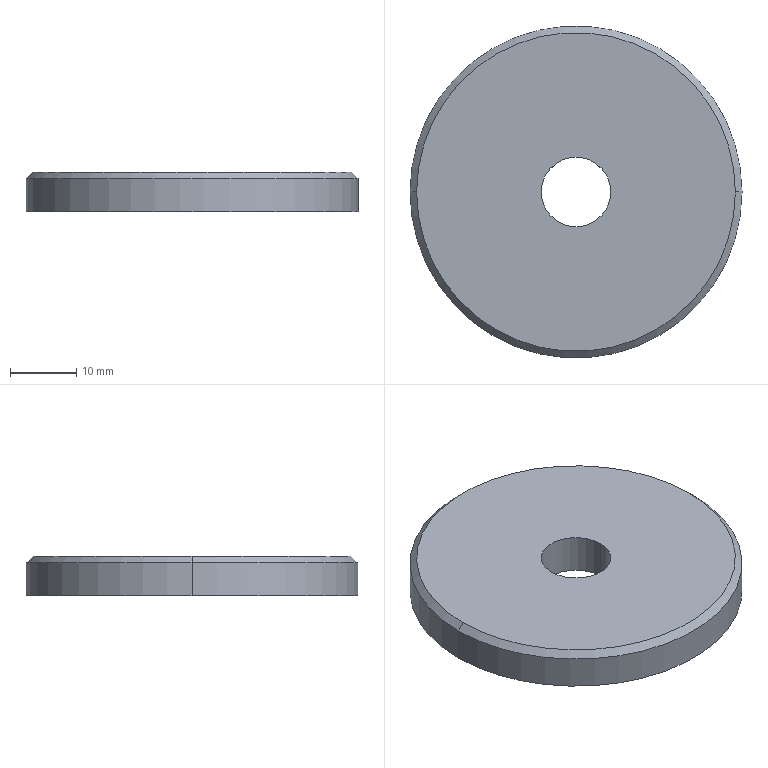Part | SolidWorks | features Chamfer 1, Extrusion 1 | 1 solid | 8 faces | box 50 x 50 x 6 mm | volume 11184 mm3 | cylinder 4 | cone 2 | plane 2 | commonest cylinder face diameters 10.5 x2 50 x2
STEP:
#1=CARTESIAN_POINT('',(24.,0.,6.));
#2=VERTEX_POINT('',#1);
#3=CARTESIAN_POINT('',(-24.,0.,6.));
#4=VERTEX_POINT('',#3);
#5=CARTESIAN_POINT('',(0.,0.,6.));
#6=DIRECTION('',(0.,0.,1.));
#7=DIRECTION('',(1.,0.,0.));
#8=AXIS2_PLACEMENT_3D('',#5,#6,#7);
#9=CIRCLE('',#8,24.);
#10=EDGE_CURVE('',#2,#4,#9,.T.);
#11=ORIENTED_EDGE('',*,*,#10,.F.);
#12=CARTESIAN_POINT('',(25.,0.,5.));
#13=VERTEX_POINT('',#12);
#14=CARTESIAN_POINT('',(24.,0.,6.));
#15=DIRECTION('',(0.7071,0.,-0.7071));
#16=VECTOR('',#15,1000.);
#17=LINE('',#14,#16);
#18=EDGE_CURVE('',#2,#13,#17,.T.);
#19=ORIENTED_EDGE('',*,*,#18,.T.);
#20=CARTESIAN_POINT('',(-25.,0.,5.));
#21=VERTEX_POINT('',#20);
#22=CARTESIAN_POINT('',(0.,0.,5.));
#23=DIRECTION('',(0.,0.,-1.));
#24=DIRECTION('',(1.,0.,0.));
#25=AXIS2_PLACEMENT_3D('',#22,#23,#24);
#26=CIRCLE('',#25,25.);
#27=EDGE_CURVE('',#21,#13,#26,.T.);
#28=ORIENTED_EDGE('',*,*,#27,.F.);
#29=CARTESIAN_POINT('',(-24.,0.,6.));
#30=DIRECTION('',(-0.7071,0.,-0.7071));
#31=VECTOR('',#30,1000.);
#32=LINE('',#29,#31);
#33=EDGE_CURVE('',#4,#21,#32,.T.);
#34=ORIENTED_EDGE('',*,*,#33,.F.);
#35=EDGE_LOOP('',(#11,#19,#28,#34));
#36=FACE_OUTER_BOUND('',#35,.T.);
#37=CARTESIAN_POINT('',(0.,0.,6.));
#38=DIRECTION('',(0.,0.,-1.));
#39=DIRECTION('',(-1.,0.,0.));
#40=AXIS2_PLACEMENT_3D('',#37,#38,#39);
#41=CONICAL_SURFACE('',#40,24.,0.7854);
#42=ADVANCED_FACE('',(#36),#41,.T.);
#43=CARTESIAN_POINT('',(-5.25,0.,6.));
#44=VERTEX_POINT('',#43);
#45=CARTESIAN_POINT('',(5.25,0.,6.));
#46=VERTEX_POINT('',#45);
#47=CARTESIAN_POINT('',(0.,0.,6.));
#48=DIRECTION('',(0.,0.,1.));
#49=DIRECTION('',(1.,0.,0.));
#50=AXIS2_PLACEMENT_3D('',#47,#48,#49);
#51=CIRCLE('',#50,5.25);
#52=EDGE_CURVE('',#44,#46,#51,.T.);
#53=ORIENTED_EDGE('',*,*,#52,.T.);
#54=CARTESIAN_POINT('',(5.25,0.,0.));
#55=VERTEX_POINT('',#54);
#56=CARTESIAN_POINT('',(5.25,0.,6.));
#57=DIRECTION('',(0.,0.,-1.));
#58=VECTOR('',#57,1000.);
#59=LINE('',#56,#58);
#60=EDGE_CURVE('',#46,#55,#59,.T.);
#61=ORIENTED_EDGE('',*,*,#60,.T.);
#62=CARTESIAN_POINT('',(-5.25,0.,0.));
#63=VERTEX_POINT('',#62);
#64=CARTESIAN_POINT('',(0.,0.,0.));
#65=DIRECTION('',(0.,0.,1.));
#66=DIRECTION('',(1.,0.,0.));
#67=AXIS2_PLACEMENT_3D('',#64,#65,#66);
#68=CIRCLE('',#67,5.25);
#69=EDGE_CURVE('',#63,#55,#68,.T.);
#70=ORIENTED_EDGE('',*,*,#69,.F.);
#71=CARTESIAN_POINT('',(-5.25,0.,6.));
#72=DIRECTION('',(0.,0.,-1.));
#73=VECTOR('',#72,1000.);
#74=LINE('',#71,#73);
#75=EDGE_CURVE('',#44,#63,#74,.T.);
#76=ORIENTED_EDGE('',*,*,#75,.F.);
#77=EDGE_LOOP('',(#53,#61,#70,#76));
#78=FACE_OUTER_BOUND('',#77,.T.);
#79=CARTESIAN_POINT('',(0.,0.,6.));
#80=DIRECTION('',(0.,0.,-1.));
#81=DIRECTION('',(-1.,0.,0.));
#82=AXIS2_PLACEMENT_3D('',#79,#80,#81);
#83=CYLINDRICAL_SURFACE('',#82,5.25);
#84=ADVANCED_FACE('',(#78),#83,.F.);
#85=ORIENTED_EDGE('',*,*,#27,.T.);
#86=CARTESIAN_POINT('',(25.,0.,0.));
#87=VERTEX_POINT('',#86);
#88=CARTESIAN_POINT('',(25.,0.,6.));
#89=DIRECTION('',(0.,0.,-1.));
#90=VECTOR('',#89,1000.);
#91=LINE('',#88,#90);
#92=EDGE_CURVE('',#13,#87,#91,.T.);
#93=ORIENTED_EDGE('',*,*,#92,.T.);
#94=CARTESIAN_POINT('',(-25.,0.,0.));
#95=VERTEX_POINT('',#94);
#96=CARTESIAN_POINT('',(0.,0.,0.));
#97=DIRECTION('',(0.,0.,1.));
#98=DIRECTION('',(1.,0.,0.));
#99=AXIS2_PLACEMENT_3D('',#96,#97,#98);
#100=CIRCLE('',#99,25.);
#101=EDGE_CURVE('',#87,#95,#100,.T.);
#102=ORIENTED_EDGE('',*,*,#101,.T.);
#103=CARTESIAN_POINT('',(-25.,0.,6.));
#104=DIRECTION('',(0.,0.,-1.));
#105=VECTOR('',#104,1000.);
#106=LINE('',#103,#105);
#107=EDGE_CURVE('',#21,#95,#106,.T.);
#108=ORIENTED_EDGE('',*,*,#107,.F.);
#109=EDGE_LOOP('',(#85,#93,#102,#108));
#110=FACE_OUTER_BOUND('',#109,.T.);
#111=CARTESIAN_POINT('',(0.,0.,6.));
#112=DIRECTION('',(0.,0.,-1.));
#113=DIRECTION('',(-1.,0.,0.));
#114=AXIS2_PLACEMENT_3D('',#111,#112,#113);
#115=CYLINDRICAL_SURFACE('',#114,25.);
#116=ADVANCED_FACE('',(#110),#115,.T.);
#117=CARTESIAN_POINT('',(0.,0.,6.));
#118=DIRECTION('',(0.,0.,1.));
#119=DIRECTION('',(1.,0.,0.));
#120=AXIS2_PLACEMENT_3D('',#117,#118,#119);
#121=CIRCLE('',#120,24.);
#122=EDGE_CURVE('',#4,#2,#121,.T.);
#123=ORIENTED_EDGE('',*,*,#122,.T.);
#124=ORIENTED_EDGE('',*,*,#10,.T.);
#125=EDGE_LOOP('',(#123,#124));
#126=FACE_OUTER_BOUND('',#125,.T.);
#127=ORIENTED_EDGE('',*,*,#52,.F.);
#128=CARTESIAN_POINT('',(0.,0.,6.));
#129=DIRECTION('',(0.,0.,1.));
#130=DIRECTION('',(1.,0.,0.));
#131=AXIS2_PLACEMENT_3D('',#128,#129,#130);
#132=CIRCLE('',#131,5.25);
#133=EDGE_CURVE('',#46,#44,#132,.T.);
#134=ORIENTED_EDGE('',*,*,#133,.F.);
#135=EDGE_LOOP('',(#127,#134));
#136=FACE_BOUND('',#135,.T.);
#137=CARTESIAN_POINT('',(0.,0.,6.));
#138=DIRECTION('',(0.,0.,1.));
#139=DIRECTION('',(1.,0.,0.));
#140=AXIS2_PLACEMENT_3D('',#137,#138,#139);
#141=PLANE('',#140);
#142=ADVANCED_FACE('',(#126,#136),#141,.T.);
#143=CARTESIAN_POINT('',(0.,0.,0.));
#144=DIRECTION('',(0.,0.,1.));
#145=DIRECTION('',(1.,0.,0.));
#146=AXIS2_PLACEMENT_3D('',#143,#144,#145);
#147=CIRCLE('',#146,25.);
#148=EDGE_CURVE('',#95,#87,#147,.T.);
#149=ORIENTED_EDGE('',*,*,#148,.F.);
#150=ORIENTED_EDGE('',*,*,#101,.F.);
#151=EDGE_LOOP('',(#149,#150));
#152=FACE_OUTER_BOUND('',#151,.T.);
#153=ORIENTED_EDGE('',*,*,#69,.T.);
#154=CARTESIAN_POINT('',(0.,0.,0.));
#155=DIRECTION('',(0.,0.,1.));
#156=DIRECTION('',(1.,0.,0.));
#157=AXIS2_PLACEMENT_3D('',#154,#155,#156);
#158=CIRCLE('',#157,5.25);
#159=EDGE_CURVE('',#55,#63,#158,.T.);
#160=ORIENTED_EDGE('',*,*,#159,.T.);
#161=EDGE_LOOP('',(#153,#160));
#162=FACE_BOUND('',#161,.T.);
#163=CARTESIAN_POINT('',(0.,0.,0.));
#164=DIRECTION('',(0.,0.,1.));
#165=DIRECTION('',(1.,0.,0.));
#166=AXIS2_PLACEMENT_3D('',#163,#164,#165);
#167=PLANE('',#166);
#168=ADVANCED_FACE('',(#152,#162),#167,.F.);
#169=ORIENTED_EDGE('',*,*,#92,.F.);
#170=CARTESIAN_POINT('',(0.,0.,5.));
#171=DIRECTION('',(0.,0.,-1.));
#172=DIRECTION('',(1.,0.,0.));
#173=AXIS2_PLACEMENT_3D('',#170,#171,#172);
#174=CIRCLE('',#173,25.);
#175=EDGE_CURVE('',#13,#21,#174,.T.);
#176=ORIENTED_EDGE('',*,*,#175,.T.);
#177=ORIENTED_EDGE('',*,*,#107,.T.);
#178=ORIENTED_EDGE('',*,*,#148,.T.);
#179=EDGE_LOOP('',(#169,#176,#177,#178));
#180=FACE_OUTER_BOUND('',#179,.T.);
#181=CARTESIAN_POINT('',(0.,0.,6.));
#182=DIRECTION('',(0.,0.,-1.));
#183=DIRECTION('',(-1.,0.,0.));
#184=AXIS2_PLACEMENT_3D('',#181,#182,#183);
#185=CYLINDRICAL_SURFACE('',#184,25.);
#186=ADVANCED_FACE('',(#180),#185,.T.);
#187=ORIENTED_EDGE('',*,*,#60,.F.);
#188=ORIENTED_EDGE('',*,*,#133,.T.);
#189=ORIENTED_EDGE('',*,*,#75,.T.);
#190=ORIENTED_EDGE('',*,*,#159,.F.);
#191=EDGE_LOOP('',(#187,#188,#189,#190));
#192=FACE_OUTER_BOUND('',#191,.T.);
#193=CARTESIAN_POINT('',(0.,0.,6.));
#194=DIRECTION('',(0.,0.,-1.));
#195=DIRECTION('',(-1.,0.,0.));
#196=AXIS2_PLACEMENT_3D('',#193,#194,#195);
#197=CYLINDRICAL_SURFACE('',#196,5.25);
#198=ADVANCED_FACE('',(#192),#197,.F.);
#199=ORIENTED_EDGE('',*,*,#18,.F.);
#200=ORIENTED_EDGE('',*,*,#122,.F.);
#201=ORIENTED_EDGE('',*,*,#33,.T.);
#202=ORIENTED_EDGE('',*,*,#175,.F.);
#203=EDGE_LOOP('',(#199,#200,#201,#202));
#204=FACE_OUTER_BOUND('',#203,.T.);
#205=CARTESIAN_POINT('',(0.,0.,6.));
#206=DIRECTION('',(0.,0.,-1.));
#207=DIRECTION('',(-1.,0.,0.));
#208=AXIS2_PLACEMENT_3D('',#205,#206,#207);
#209=CONICAL_SURFACE('',#208,24.,0.7854);
#210=ADVANCED_FACE('',(#204),#209,.T.);
#211=CLOSED_SHELL('',(#42,#84,#116,#142,#168,#186,#198,#210));
#212=MANIFOLD_SOLID_BREP('',#211);
#213=CARTESIAN_POINT('',(0.,0.,0.));
#214=DIRECTION('',(0.,0.,1.));
#215=DIRECTION('',(1.,0.,0.));
#216=AXIS2_PLACEMENT_3D('',#213,#214,#215);
#217=(LENGTH_UNIT()NAMED_UNIT(*)SI_UNIT(.MILLI.,.METRE.));
#218=UNCERTAINTY_MEASURE_WITH_UNIT(LENGTH_MEASURE(0.00001),#217,'','');
#219=(NAMED_UNIT(*)PLANE_ANGLE_UNIT()SI_UNIT($,.RADIAN.));
#220=(NAMED_UNIT(*)SI_UNIT($,.STERADIAN.)SOLID_ANGLE_UNIT());
#221=(GEOMETRIC_REPRESENTATION_CONTEXT(3)GLOBAL_UNCERTAINTY_ASSIGNED_CONTEXT((#218))GLOBAL_UNIT_ASSIGNED_CONTEXT((#217,#219,#220))REPRESENTATION_CONTEXT('',''));
#222=ADVANCED_BREP_SHAPE_REPRESENTATION('',(#212,#216),#221);